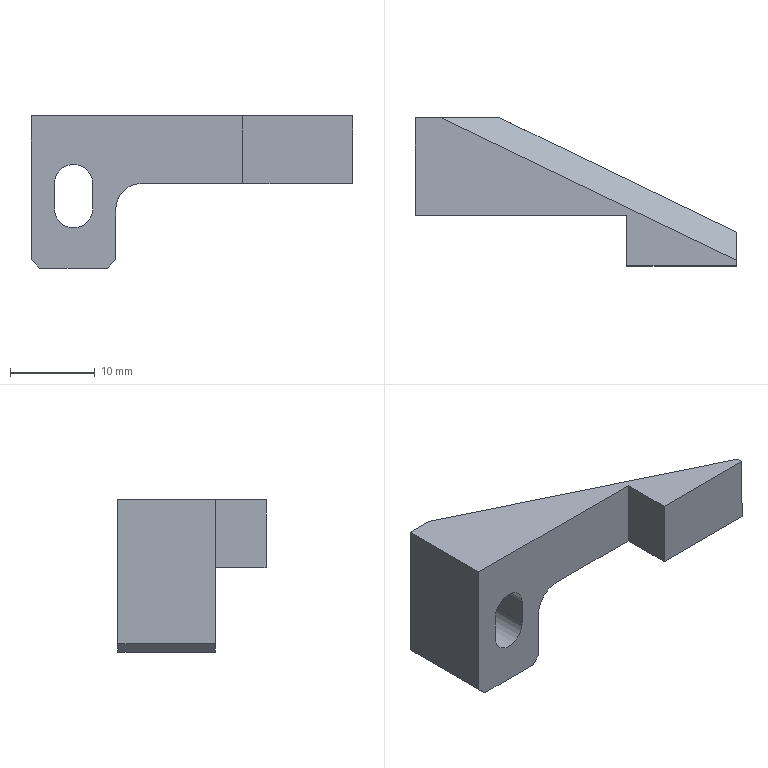Part | SolidWorks | features ICE 4, Chamfer 2, Extrusion 1, Fillet 1 | 1 solid | 25 faces | box 38 x 17.5 x 18 mm | volume 3099 mm3 | plane 19 | cylinder 6 | commonest cylinder face diameters 8 x3 4.5 x2 6 x1
STEP:
#1=CARTESIAN_POINT('',(5.,13.5,14.));
#2=VERTEX_POINT('',#1);
#3=CARTESIAN_POINT('',(9.,13.5,10.));
#4=VERTEX_POINT('',#3);
#5=CARTESIAN_POINT('',(5.,13.5,10.));
#6=DIRECTION('',(0.,1.,0.));
#7=DIRECTION('',(0.,0.,1.));
#8=AXIS2_PLACEMENT_3D('',#5,#6,#7);
#9=CIRCLE('',#8,4.);
#10=EDGE_CURVE('',#2,#4,#9,.T.);
#11=ORIENTED_EDGE('',*,*,#10,.F.);
#12=CARTESIAN_POINT('',(5.,17.5,14.));
#13=VERTEX_POINT('',#12);
#14=CARTESIAN_POINT('',(5.,13.5,14.));
#15=DIRECTION('',(0.,1.,0.));
#16=VECTOR('',#15,1000.);
#17=LINE('',#14,#16);
#18=EDGE_CURVE('',#2,#13,#17,.T.);
#19=ORIENTED_EDGE('',*,*,#18,.T.);
#20=CARTESIAN_POINT('',(9.,17.5,10.));
#21=VERTEX_POINT('',#20);
#22=CARTESIAN_POINT('',(5.,17.5,10.));
#23=DIRECTION('',(0.,1.,0.));
#24=DIRECTION('',(0.,0.,1.));
#25=AXIS2_PLACEMENT_3D('',#22,#23,#24);
#26=CIRCLE('',#25,4.);
#27=EDGE_CURVE('',#13,#21,#26,.T.);
#28=ORIENTED_EDGE('',*,*,#27,.T.);
#29=CARTESIAN_POINT('',(9.,13.5,10.));
#30=DIRECTION('',(0.,1.,0.));
#31=VECTOR('',#30,1000.);
#32=LINE('',#29,#31);
#33=EDGE_CURVE('',#4,#21,#32,.T.);
#34=ORIENTED_EDGE('',*,*,#33,.F.);
#35=EDGE_LOOP('',(#11,#19,#28,#34));
#36=FACE_OUTER_BOUND('',#35,.T.);
#37=CARTESIAN_POINT('',(5.,13.5,10.));
#38=DIRECTION('',(0.,1.,0.));
#39=DIRECTION('',(0.,0.,1.));
#40=AXIS2_PLACEMENT_3D('',#37,#38,#39);
#41=CYLINDRICAL_SURFACE('',#40,4.);
#42=ADVANCED_FACE('',(#36),#41,.F.);
#43=CARTESIAN_POINT('',(7.25,6.,10.));
#44=VERTEX_POINT('',#43);
#45=CARTESIAN_POINT('',(7.25,13.5,10.));
#46=VERTEX_POINT('',#45);
#47=CARTESIAN_POINT('',(7.25,-2.5,10.));
#48=DIRECTION('',(0.,1.,0.));
#49=VECTOR('',#48,1000.);
#50=LINE('',#47,#49);
#51=EDGE_CURVE('',#44,#46,#50,.T.);
#52=ORIENTED_EDGE('',*,*,#51,.F.);
#53=CARTESIAN_POINT('',(2.75,6.,10.));
#54=VERTEX_POINT('',#53);
#55=CARTESIAN_POINT('',(5.,6.,10.));
#56=DIRECTION('',(0.,-1.,0.));
#57=DIRECTION('',(0.,0.,1.));
#58=AXIS2_PLACEMENT_3D('',#55,#56,#57);
#59=CIRCLE('',#58,2.25);
#60=EDGE_CURVE('',#44,#54,#59,.T.);
#61=ORIENTED_EDGE('',*,*,#60,.T.);
#62=CARTESIAN_POINT('',(2.75,13.5,10.));
#63=VERTEX_POINT('',#62);
#64=CARTESIAN_POINT('',(2.75,-2.5,10.));
#65=DIRECTION('',(0.,1.,0.));
#66=VECTOR('',#65,1000.);
#67=LINE('',#64,#66);
#68=EDGE_CURVE('',#54,#63,#67,.T.);
#69=ORIENTED_EDGE('',*,*,#68,.T.);
#70=CARTESIAN_POINT('',(5.,13.5,10.));
#71=DIRECTION('',(0.,-1.,0.));
#72=DIRECTION('',(0.,0.,1.));
#73=AXIS2_PLACEMENT_3D('',#70,#71,#72);
#74=CIRCLE('',#73,2.25);
#75=EDGE_CURVE('',#46,#63,#74,.T.);
#76=ORIENTED_EDGE('',*,*,#75,.F.);
#77=EDGE_LOOP('',(#52,#61,#69,#76));
#78=FACE_OUTER_BOUND('',#77,.T.);
#79=CARTESIAN_POINT('',(5.,-2.5,10.));
#80=DIRECTION('',(0.,1.,0.));
#81=DIRECTION('',(-1.,0.,0.));
#82=AXIS2_PLACEMENT_3D('',#79,#80,#81);
#83=CYLINDRICAL_SURFACE('',#82,2.25);
#84=ADVANCED_FACE('',(#78),#83,.F.);
#85=ORIENTED_EDGE('',*,*,#68,.F.);
#86=CARTESIAN_POINT('',(2.75,6.,7.));
#87=VERTEX_POINT('',#86);
#88=CARTESIAN_POINT('',(2.75,6.,10.));
#89=DIRECTION('',(0.,0.,-1.));
#90=VECTOR('',#89,1000.);
#91=LINE('',#88,#90);
#92=EDGE_CURVE('',#54,#87,#91,.T.);
#93=ORIENTED_EDGE('',*,*,#92,.T.);
#94=CARTESIAN_POINT('',(2.75,13.5,7.));
#95=VERTEX_POINT('',#94);
#96=CARTESIAN_POINT('',(2.75,-2.5,7.));
#97=DIRECTION('',(0.,1.,0.));
#98=VECTOR('',#97,1000.);
#99=LINE('',#96,#98);
#100=EDGE_CURVE('',#87,#95,#99,.T.);
#101=ORIENTED_EDGE('',*,*,#100,.T.);
#102=CARTESIAN_POINT('',(2.75,13.5,10.));
#103=DIRECTION('',(0.,0.,-1.));
#104=VECTOR('',#103,1000.);
#105=LINE('',#102,#104);
#106=EDGE_CURVE('',#63,#95,#105,.T.);
#107=ORIENTED_EDGE('',*,*,#106,.F.);
#108=EDGE_LOOP('',(#85,#93,#101,#107));
#109=FACE_OUTER_BOUND('',#108,.T.);
#110=CARTESIAN_POINT('',(2.75,-2.5,10.));
#111=DIRECTION('',(-1.,0.,0.));
#112=DIRECTION('',(0.,-1.,0.));
#113=AXIS2_PLACEMENT_3D('',#110,#111,#112);
#114=PLANE('',#113);
#115=ADVANCED_FACE('',(#109),#114,.F.);
#116=ORIENTED_EDGE('',*,*,#100,.F.);
#117=CARTESIAN_POINT('',(7.25,6.,7.));
#118=VERTEX_POINT('',#117);
#119=CARTESIAN_POINT('',(5.,6.,7.));
#120=DIRECTION('',(0.,-1.,0.));
#121=DIRECTION('',(0.,0.,1.));
#122=AXIS2_PLACEMENT_3D('',#119,#120,#121);
#123=CIRCLE('',#122,2.25);
#124=EDGE_CURVE('',#87,#118,#123,.T.);
#125=ORIENTED_EDGE('',*,*,#124,.T.);
#126=CARTESIAN_POINT('',(7.25,13.5,7.));
#127=VERTEX_POINT('',#126);
#128=CARTESIAN_POINT('',(7.25,-2.5,7.));
#129=DIRECTION('',(0.,1.,0.));
#130=VECTOR('',#129,1000.);
#131=LINE('',#128,#130);
#132=EDGE_CURVE('',#118,#127,#131,.T.);
#133=ORIENTED_EDGE('',*,*,#132,.T.);
#134=CARTESIAN_POINT('',(5.,13.5,7.));
#135=DIRECTION('',(0.,-1.,0.));
#136=DIRECTION('',(0.,0.,1.));
#137=AXIS2_PLACEMENT_3D('',#134,#135,#136);
#138=CIRCLE('',#137,2.25);
#139=EDGE_CURVE('',#95,#127,#138,.T.);
#140=ORIENTED_EDGE('',*,*,#139,.F.);
#141=EDGE_LOOP('',(#116,#125,#133,#140));
#142=FACE_OUTER_BOUND('',#141,.T.);
#143=CARTESIAN_POINT('',(5.,-2.5,7.));
#144=DIRECTION('',(0.,1.,0.));
#145=DIRECTION('',(-1.,0.,0.));
#146=AXIS2_PLACEMENT_3D('',#143,#144,#145);
#147=CYLINDRICAL_SURFACE('',#146,2.25);
#148=ADVANCED_FACE('',(#142),#147,.F.);
#149=ORIENTED_EDGE('',*,*,#132,.F.);
#150=CARTESIAN_POINT('',(7.25,6.,10.));
#151=DIRECTION('',(0.,0.,1.));
#152=VECTOR('',#151,1000.);
#153=LINE('',#150,#152);
#154=EDGE_CURVE('',#118,#44,#153,.T.);
#155=ORIENTED_EDGE('',*,*,#154,.T.);
#156=ORIENTED_EDGE('',*,*,#51,.T.);
#157=CARTESIAN_POINT('',(7.25,13.5,10.));
#158=DIRECTION('',(0.,0.,1.));
#159=VECTOR('',#158,1000.);
#160=LINE('',#157,#159);
#161=EDGE_CURVE('',#127,#46,#160,.T.);
#162=ORIENTED_EDGE('',*,*,#161,.F.);
#163=EDGE_LOOP('',(#149,#155,#156,#162));
#164=FACE_OUTER_BOUND('',#163,.T.);
#165=CARTESIAN_POINT('',(7.25,-2.5,10.));
#166=DIRECTION('',(1.,0.,0.));
#167=DIRECTION('',(0.,1.,0.));
#168=AXIS2_PLACEMENT_3D('',#165,#166,#167);
#169=PLANE('',#168);
#170=ADVANCED_FACE('',(#164),#169,.F.);
#171=CARTESIAN_POINT('',(1.,17.5,7.));
#172=VERTEX_POINT('',#171);
#173=CARTESIAN_POINT('',(1.,17.5,10.));
#174=VERTEX_POINT('',#173);
#175=CARTESIAN_POINT('',(1.,17.5,7.));
#176=DIRECTION('',(0.,0.,1.));
#177=VECTOR('',#176,1000.);
#178=LINE('',#175,#177);
#179=EDGE_CURVE('',#172,#174,#178,.T.);
#180=ORIENTED_EDGE('',*,*,#179,.F.);
#181=CARTESIAN_POINT('',(9.,17.5,7.));
#182=VERTEX_POINT('',#181);
#183=CARTESIAN_POINT('',(5.,17.5,7.));
#184=DIRECTION('',(0.,1.,0.));
#185=DIRECTION('',(0.,0.,1.));
#186=AXIS2_PLACEMENT_3D('',#183,#184,#185);
#187=CIRCLE('',#186,4.);
#188=EDGE_CURVE('',#182,#172,#187,.T.);
#189=ORIENTED_EDGE('',*,*,#188,.F.);
#190=CARTESIAN_POINT('',(9.,17.5,7.));
#191=DIRECTION('',(0.,0.,-1.));
#192=VECTOR('',#191,1000.);
#193=LINE('',#190,#192);
#194=EDGE_CURVE('',#21,#182,#193,.T.);
#195=ORIENTED_EDGE('',*,*,#194,.F.);
#196=ORIENTED_EDGE('',*,*,#27,.F.);
#197=CARTESIAN_POINT('',(5.,17.5,10.));
#198=DIRECTION('',(0.,1.,0.));
#199=DIRECTION('',(0.,0.,1.));
#200=AXIS2_PLACEMENT_3D('',#197,#198,#199);
#201=CIRCLE('',#200,4.);
#202=EDGE_CURVE('',#174,#13,#201,.T.);
#203=ORIENTED_EDGE('',*,*,#202,.F.);
#204=EDGE_LOOP('',(#180,#189,#195,#196,#203));
#205=FACE_BOUND('',#204,.T.);
#206=CARTESIAN_POINT('',(9.,17.5,0.));
#207=VERTEX_POINT('',#206);
#208=CARTESIAN_POINT('',(1.,17.5,0.));
#209=VERTEX_POINT('',#208);
#210=CARTESIAN_POINT('',(10.,17.5,0.));
#211=DIRECTION('',(-1.,0.,0.));
#212=VECTOR('',#211,1000.);
#213=LINE('',#210,#212);
#214=EDGE_CURVE('',#207,#209,#213,.T.);
#215=ORIENTED_EDGE('',*,*,#214,.T.);
#216=CARTESIAN_POINT('',(0.,17.5,1.));
#217=VERTEX_POINT('',#216);
#218=CARTESIAN_POINT('',(0.,17.5,1.));
#219=DIRECTION('',(-0.7071,0.,0.7071));
#220=VECTOR('',#219,1000.);
#221=LINE('',#218,#220);
#222=EDGE_CURVE('',#209,#217,#221,.T.);
#223=ORIENTED_EDGE('',*,*,#222,.T.);
#224=CARTESIAN_POINT('',(0.,17.5,18.));
#225=VERTEX_POINT('',#224);
#226=CARTESIAN_POINT('',(0.,17.5,18.));
#227=DIRECTION('',(0.,0.,-1.));
#228=VECTOR('',#227,1000.);
#229=LINE('',#226,#228);
#230=EDGE_CURVE('',#225,#217,#229,.T.);
#231=ORIENTED_EDGE('',*,*,#230,.F.);
#232=CARTESIAN_POINT('',(3.092,17.5,18.));
#233=VERTEX_POINT('',#232);
#234=CARTESIAN_POINT('',(10.,17.5,18.));
#235=DIRECTION('',(-1.,0.,0.));
#236=VECTOR('',#235,1000.);
#237=LINE('',#234,#236);
#238=EDGE_CURVE('',#233,#225,#237,.T.);
#239=ORIENTED_EDGE('',*,*,#238,.F.);
#240=CARTESIAN_POINT('',(10.,17.5,15.));
#241=VERTEX_POINT('',#240);
#242=CARTESIAN_POINT('',(0.9814,17.5,18.917));
#243=DIRECTION('',(0.9172,0.,-0.3984));
#244=VECTOR('',#243,1000.);
#245=LINE('',#242,#244);
#246=EDGE_CURVE('',#233,#241,#245,.T.);
#247=ORIENTED_EDGE('',*,*,#246,.T.);
#248=CARTESIAN_POINT('',(10.,17.5,7.));
#249=VERTEX_POINT('',#248);
#250=CARTESIAN_POINT('',(10.,17.5,18.));
#251=DIRECTION('',(0.,0.,-1.));
#252=VECTOR('',#251,1000.);
#253=LINE('',#250,#252);
#254=EDGE_CURVE('',#241,#249,#253,.T.);
#255=ORIENTED_EDGE('',*,*,#254,.T.);
#256=CARTESIAN_POINT('',(10.,17.5,1.));
#257=VERTEX_POINT('',#256);
#258=CARTESIAN_POINT('',(10.,17.5,0.));
#259=DIRECTION('',(0.,0.,1.));
#260=VECTOR('',#259,1000.);
#261=LINE('',#258,#260);
#262=EDGE_CURVE('',#257,#249,#261,.T.);
#263=ORIENTED_EDGE('',*,*,#262,.F.);
#264=CARTESIAN_POINT('',(10.,17.5,1.));
#265=DIRECTION('',(-0.7071,0.,-0.7071));
#266=VECTOR('',#265,1000.);
#267=LINE('',#264,#266);
#268=EDGE_CURVE('',#257,#207,#267,.T.);
#269=ORIENTED_EDGE('',*,*,#268,.T.);
#270=EDGE_LOOP('',(#215,#223,#231,#239,#247,#255,#263,#269));
#271=FACE_OUTER_BOUND('',#270,.T.);
#272=CARTESIAN_POINT('',(10.,17.5,18.));
#273=DIRECTION('',(0.,-1.,0.));
#274=DIRECTION('',(1.,0.,0.));
#275=AXIS2_PLACEMENT_3D('',#272,#273,#274);
#276=PLANE('',#275);
#277=ADVANCED_FACE('',(#205,#271),#276,.F.);
#278=ORIENTED_EDGE('',*,*,#230,.T.);
#279=CARTESIAN_POINT('',(0.,6.,1.));
#280=VERTEX_POINT('',#279);
#281=CARTESIAN_POINT('',(0.,17.5,1.));
#282=DIRECTION('',(0.,-1.,0.));
#283=VECTOR('',#282,1000.);
#284=LINE('',#281,#283);
#285=EDGE_CURVE('',#217,#280,#284,.T.);
#286=ORIENTED_EDGE('',*,*,#285,.T.);
#287=CARTESIAN_POINT('',(0.,6.,18.));
#288=VERTEX_POINT('',#287);
#289=CARTESIAN_POINT('',(0.,6.,0.));
#290=DIRECTION('',(0.,0.,1.));
#291=VECTOR('',#290,1000.);
#292=LINE('',#289,#291);
#293=EDGE_CURVE('',#280,#288,#292,.T.);
#294=ORIENTED_EDGE('',*,*,#293,.T.);
#295=CARTESIAN_POINT('',(0.,17.5,18.));
#296=DIRECTION('',(0.,-1.,0.));
#297=VECTOR('',#296,1000.);
#298=LINE('',#295,#297);
#299=EDGE_CURVE('',#225,#288,#298,.T.);
#300=ORIENTED_EDGE('',*,*,#299,.F.);
#301=EDGE_LOOP('',(#278,#286,#294,#300));
#302=FACE_OUTER_BOUND('',#301,.T.);
#303=CARTESIAN_POINT('',(0.,17.5,18.));
#304=DIRECTION('',(1.,0.,0.));
#305=DIRECTION('',(0.,1.,0.));
#306=AXIS2_PLACEMENT_3D('',#303,#304,#305);
#307=PLANE('',#306);
#308=ADVANCED_FACE('',(#302),#307,.F.);
#309=CARTESIAN_POINT('',(25.,0.,10.));
#310=VERTEX_POINT('',#309);
#311=CARTESIAN_POINT('',(25.,0.,18.));
#312=VERTEX_POINT('',#311);
#313=CARTESIAN_POINT('',(25.,0.,0.));
#314=DIRECTION('',(0.,0.,1.));
#315=VECTOR('',#314,1000.);
#316=LINE('',#313,#315);
#317=EDGE_CURVE('',#310,#312,#316,.T.);
#318=ORIENTED_EDGE('',*,*,#317,.F.);
#319=CARTESIAN_POINT('',(38.,0.,10.));
#320=VERTEX_POINT('',#319);
#321=CARTESIAN_POINT('',(38.,0.,10.));
#322=DIRECTION('',(1.,0.,0.));
#323=VECTOR('',#322,1000.);
#324=LINE('',#321,#323);
#325=EDGE_CURVE('',#310,#320,#324,.T.);
#326=ORIENTED_EDGE('',*,*,#325,.T.);
#327=CARTESIAN_POINT('',(38.,0.,18.));
#328=VERTEX_POINT('',#327);
#329=CARTESIAN_POINT('',(38.,0.,18.));
#330=DIRECTION('',(0.,0.,-1.));
#331=VECTOR('',#330,1000.);
#332=LINE('',#329,#331);
#333=EDGE_CURVE('',#328,#320,#332,.T.);
#334=ORIENTED_EDGE('',*,*,#333,.F.);
#335=CARTESIAN_POINT('',(0.,0.,18.));
#336=DIRECTION('',(1.,0.,0.));
#337=VECTOR('',#336,1000.);
#338=LINE('',#335,#337);
#339=EDGE_CURVE('',#312,#328,#338,.T.);
#340=ORIENTED_EDGE('',*,*,#339,.F.);
#341=EDGE_LOOP('',(#318,#326,#334,#340));
#342=FACE_OUTER_BOUND('',#341,.T.);
#343=CARTESIAN_POINT('',(0.,0.,18.));
#344=DIRECTION('',(0.,1.,0.));
#345=DIRECTION('',(0.,0.,1.));
#346=AXIS2_PLACEMENT_3D('',#343,#344,#345);
#347=PLANE('',#346);
#348=ADVANCED_FACE('',(#342),#347,.F.);
#349=ORIENTED_EDGE('',*,*,#333,.T.);
#350=CARTESIAN_POINT('',(38.,4.,10.));
#351=VERTEX_POINT('',#350);
#352=CARTESIAN_POINT('',(38.,0.,10.));
#353=DIRECTION('',(0.,1.,0.));
#354=VECTOR('',#353,1000.);
#355=LINE('',#352,#354);
#356=EDGE_CURVE('',#320,#351,#355,.T.);
#357=ORIENTED_EDGE('',*,*,#356,.T.);
#358=CARTESIAN_POINT('',(38.,4.,15.));
#359=VERTEX_POINT('',#358);
#360=CARTESIAN_POINT('',(38.,4.,18.));
#361=DIRECTION('',(0.,0.,-1.));
#362=VECTOR('',#361,1000.);
#363=LINE('',#360,#362);
#364=EDGE_CURVE('',#359,#351,#363,.T.);
#365=ORIENTED_EDGE('',*,*,#364,.F.);
#366=CARTESIAN_POINT('',(38.,0.6695,18.));
#367=VERTEX_POINT('',#366);
#368=CARTESIAN_POINT('',(38.,10.629,9.029));
#369=DIRECTION('',(0.,-0.743,0.6693));
#370=VECTOR('',#369,1000.);
#371=LINE('',#368,#370);
#372=EDGE_CURVE('',#359,#367,#371,.T.);
#373=ORIENTED_EDGE('',*,*,#372,.T.);
#374=CARTESIAN_POINT('',(38.,0.,18.));
#375=DIRECTION('',(0.,1.,0.));
#376=VECTOR('',#375,1000.);
#377=LINE('',#374,#376);
#378=EDGE_CURVE('',#328,#367,#377,.T.);
#379=ORIENTED_EDGE('',*,*,#378,.F.);
#380=EDGE_LOOP('',(#349,#357,#365,#373,#379));
#381=FACE_OUTER_BOUND('',#380,.T.);
#382=CARTESIAN_POINT('',(38.,0.,18.));
#383=DIRECTION('',(-1.,0.,0.));
#384=DIRECTION('',(0.,0.,1.));
#385=AXIS2_PLACEMENT_3D('',#382,#383,#384);
#386=PLANE('',#385);
#387=ADVANCED_FACE('',(#381),#386,.F.);
#388=ORIENTED_EDGE('',*,*,#364,.T.);
#389=CARTESIAN_POINT('',(13.,16.054,10.));
#390=VERTEX_POINT('',#389);
#391=CARTESIAN_POINT('',(38.,4.,10.));
#392=DIRECTION('',(-0.9008,0.4343,0.));
#393=VECTOR('',#392,1000.);
#394=LINE('',#391,#393);
#395=EDGE_CURVE('',#351,#390,#394,.T.);
#396=ORIENTED_EDGE('',*,*,#395,.T.);
#397=CARTESIAN_POINT('',(13.,16.054,10.));
#398=CARTESIAN_POINT('',(11.243,16.901,10.));
#399=CARTESIAN_POINT('',(10.,17.5,8.757));
#400=CARTESIAN_POINT('',(10.,17.5,7.));
#401=(BOUNDED_CURVE()B_SPLINE_CURVE(3,(#397,#398,#399,#400),.UNSPECIFIED.,.F.,.F.)B_SPLINE_CURVE_WITH_KNOTS((4,4),(1.571,3.142),.UNSPECIFIED.)CURVE()GEOMETRIC_REPRESENTATION_ITEM()RATIONAL_B_SPLINE_CURVE((1.,0.8047,0.8047,1.))REPRESENTATION_ITEM(''));
#402=EDGE_CURVE('',#390,#249,#401,.T.);
#403=ORIENTED_EDGE('',*,*,#402,.T.);
#404=ORIENTED_EDGE('',*,*,#254,.F.);
#405=CARTESIAN_POINT('',(38.,4.,15.));
#406=DIRECTION('',(0.9008,-0.4343,0.));
#407=VECTOR('',#406,1000.);
#408=LINE('',#405,#407);
#409=EDGE_CURVE('',#241,#359,#408,.T.);
#410=ORIENTED_EDGE('',*,*,#409,.T.);
#411=EDGE_LOOP('',(#388,#396,#403,#404,#410));
#412=FACE_OUTER_BOUND('',#411,.T.);
#413=CARTESIAN_POINT('',(38.,4.,18.));
#414=DIRECTION('',(-0.4343,-0.9008,0.));
#415=DIRECTION('',(0.9008,-0.4343,0.));
#416=AXIS2_PLACEMENT_3D('',#413,#414,#415);
#417=PLANE('',#416);
#418=ADVANCED_FACE('',(#412),#417,.F.);
#419=CARTESIAN_POINT('',(25.,6.,18.));
#420=VERTEX_POINT('',#419);
#421=CARTESIAN_POINT('',(0.,6.,18.));
#422=DIRECTION('',(-1.,0.,0.));
#423=VECTOR('',#422,1000.);
#424=LINE('',#421,#423);
#425=EDGE_CURVE('',#420,#288,#424,.T.);
#426=ORIENTED_EDGE('',*,*,#425,.F.);
#427=CARTESIAN_POINT('',(25.,0.,18.));
#428=DIRECTION('',(0.,1.,0.));
#429=VECTOR('',#428,1000.);
#430=LINE('',#427,#429);
#431=EDGE_CURVE('',#312,#420,#430,.T.);
#432=ORIENTED_EDGE('',*,*,#431,.F.);
#433=ORIENTED_EDGE('',*,*,#339,.T.);
#434=ORIENTED_EDGE('',*,*,#378,.T.);
#435=CARTESIAN_POINT('',(8.697,14.798,18.));
#436=DIRECTION('',(-0.9008,0.4343,0.));
#437=VECTOR('',#436,1000.);
#438=LINE('',#435,#437);
#439=EDGE_CURVE('',#367,#233,#438,.T.);
#440=ORIENTED_EDGE('',*,*,#439,.T.);
#441=ORIENTED_EDGE('',*,*,#238,.T.);
#442=ORIENTED_EDGE('',*,*,#299,.T.);
#443=EDGE_LOOP('',(#426,#432,#433,#434,#440,#441,#442));
#444=FACE_OUTER_BOUND('',#443,.T.);
#445=CARTESIAN_POINT('',(0.,17.5,18.));
#446=DIRECTION('',(0.,0.,1.));
#447=DIRECTION('',(1.,0.,0.));
#448=AXIS2_PLACEMENT_3D('',#445,#446,#447);
#449=PLANE('',#448);
#450=ADVANCED_FACE('',(#444),#449,.T.);
#451=CARTESIAN_POINT('',(9.,6.,0.));
#452=VERTEX_POINT('',#451);
#453=CARTESIAN_POINT('',(1.,6.,0.));
#454=VERTEX_POINT('',#453);
#455=CARTESIAN_POINT('',(0.,6.,0.));
#456=DIRECTION('',(-1.,0.,0.));
#457=VECTOR('',#456,1000.);
#458=LINE('',#455,#457);
#459=EDGE_CURVE('',#452,#454,#458,.T.);
#460=ORIENTED_EDGE('',*,*,#459,.T.);
#461=CARTESIAN_POINT('',(1.,17.5,0.));
#462=DIRECTION('',(0.,1.,0.));
#463=VECTOR('',#462,1000.);
#464=LINE('',#461,#463);
#465=EDGE_CURVE('',#454,#209,#464,.T.);
#466=ORIENTED_EDGE('',*,*,#465,.T.);
#467=ORIENTED_EDGE('',*,*,#214,.F.);
#468=CARTESIAN_POINT('',(9.,17.5,0.));
#469=DIRECTION('',(0.,-1.,0.));
#470=VECTOR('',#469,1000.);
#471=LINE('',#468,#470);
#472=EDGE_CURVE('',#207,#452,#471,.T.);
#473=ORIENTED_EDGE('',*,*,#472,.T.);
#474=EDGE_LOOP('',(#460,#466,#467,#473));
#475=FACE_OUTER_BOUND('',#474,.T.);
#476=CARTESIAN_POINT('',(0.,17.5,0.));
#477=DIRECTION('',(0.,0.,1.));
#478=DIRECTION('',(1.,0.,0.));
#479=AXIS2_PLACEMENT_3D('',#476,#477,#478);
#480=PLANE('',#479);
#481=ADVANCED_FACE('',(#475),#480,.F.);
#482=ORIENTED_EDGE('',*,*,#372,.F.);
#483=ORIENTED_EDGE('',*,*,#409,.F.);
#484=ORIENTED_EDGE('',*,*,#246,.F.);
#485=ORIENTED_EDGE('',*,*,#439,.F.);
#486=EDGE_LOOP('',(#482,#483,#484,#485));
#487=FACE_OUTER_BOUND('',#486,.T.);
#488=CARTESIAN_POINT('',(0.5833,18.71,18.));
#489=DIRECTION('',(0.3071,0.6369,0.7071));
#490=DIRECTION('',(0.,-0.743,0.6693));
#491=AXIS2_PLACEMENT_3D('',#488,#489,#490);
#492=PLANE('',#491);
#493=ADVANCED_FACE('',(#487),#492,.T.);
#494=CARTESIAN_POINT('',(9.,13.5,7.));
#495=VERTEX_POINT('',#494);
#496=CARTESIAN_POINT('',(1.,13.5,7.));
#497=VERTEX_POINT('',#496);
#498=CARTESIAN_POINT('',(5.,13.5,7.));
#499=DIRECTION('',(0.,1.,0.));
#500=DIRECTION('',(0.,0.,1.));
#501=AXIS2_PLACEMENT_3D('',#498,#499,#500);
#502=CIRCLE('',#501,4.);
#503=EDGE_CURVE('',#495,#497,#502,.T.);
#504=ORIENTED_EDGE('',*,*,#503,.T.);
#505=CARTESIAN_POINT('',(1.,13.5,10.));
#506=VERTEX_POINT('',#505);
#507=CARTESIAN_POINT('',(1.,13.5,7.));
#508=DIRECTION('',(0.,0.,1.));
#509=VECTOR('',#508,1000.);
#510=LINE('',#507,#509);
#511=EDGE_CURVE('',#497,#506,#510,.T.);
#512=ORIENTED_EDGE('',*,*,#511,.T.);
#513=CARTESIAN_POINT('',(5.,13.5,10.));
#514=DIRECTION('',(0.,1.,0.));
#515=DIRECTION('',(0.,0.,1.));
#516=AXIS2_PLACEMENT_3D('',#513,#514,#515);
#517=CIRCLE('',#516,4.);
#518=EDGE_CURVE('',#506,#2,#517,.T.);
#519=ORIENTED_EDGE('',*,*,#518,.T.);
#520=ORIENTED_EDGE('',*,*,#10,.T.);
#521=CARTESIAN_POINT('',(9.,13.5,7.));
#522=DIRECTION('',(0.,0.,-1.));
#523=VECTOR('',#522,1000.);
#524=LINE('',#521,#523);
#525=EDGE_CURVE('',#4,#495,#524,.T.);
#526=ORIENTED_EDGE('',*,*,#525,.T.);
#527=EDGE_LOOP('',(#504,#512,#519,#520,#526));
#528=FACE_OUTER_BOUND('',#527,.T.);
#529=ORIENTED_EDGE('',*,*,#75,.T.);
#530=ORIENTED_EDGE('',*,*,#106,.T.);
#531=ORIENTED_EDGE('',*,*,#139,.T.);
#532=ORIENTED_EDGE('',*,*,#161,.T.);
#533=EDGE_LOOP('',(#529,#530,#531,#532));
#534=FACE_BOUND('',#533,.T.);
#535=CARTESIAN_POINT('',(5.,13.5,7.));
#536=DIRECTION('',(0.,1.,0.));
#537=DIRECTION('',(0.,0.,1.));
#538=AXIS2_PLACEMENT_3D('',#535,#536,#537);
#539=PLANE('',#538);
#540=ADVANCED_FACE('',(#528,#534),#539,.T.);
#541=ORIENTED_EDGE('',*,*,#188,.T.);
#542=CARTESIAN_POINT('',(1.,13.5,7.));
#543=DIRECTION('',(0.,1.,0.));
#544=VECTOR('',#543,1000.);
#545=LINE('',#542,#544);
#546=EDGE_CURVE('',#497,#172,#545,.T.);
#547=ORIENTED_EDGE('',*,*,#546,.F.);
#548=ORIENTED_EDGE('',*,*,#503,.F.);
#549=CARTESIAN_POINT('',(9.,13.5,7.));
#550=DIRECTION('',(0.,1.,0.));
#551=VECTOR('',#550,1000.);
#552=LINE('',#549,#551);
#553=EDGE_CURVE('',#495,#182,#552,.T.);
#554=ORIENTED_EDGE('',*,*,#553,.T.);
#555=EDGE_LOOP('',(#541,#547,#548,#554));
#556=FACE_OUTER_BOUND('',#555,.T.);
#557=CARTESIAN_POINT('',(5.,13.5,7.));
#558=DIRECTION('',(0.,1.,0.));
#559=DIRECTION('',(0.,0.,1.));
#560=AXIS2_PLACEMENT_3D('',#557,#558,#559);
#561=CYLINDRICAL_SURFACE('',#560,4.);
#562=ADVANCED_FACE('',(#556),#561,.F.);
#563=ORIENTED_EDGE('',*,*,#194,.T.);
#564=ORIENTED_EDGE('',*,*,#553,.F.);
#565=ORIENTED_EDGE('',*,*,#525,.F.);
#566=ORIENTED_EDGE('',*,*,#33,.T.);
#567=EDGE_LOOP('',(#563,#564,#565,#566));
#568=FACE_OUTER_BOUND('',#567,.T.);
#569=CARTESIAN_POINT('',(9.,13.5,7.));
#570=DIRECTION('',(1.,0.,0.));
#571=DIRECTION('',(0.,0.,-1.));
#572=AXIS2_PLACEMENT_3D('',#569,#570,#571);
#573=PLANE('',#572);
#574=ADVANCED_FACE('',(#568),#573,.F.);
#575=ORIENTED_EDGE('',*,*,#18,.F.);
#576=ORIENTED_EDGE('',*,*,#518,.F.);
#577=CARTESIAN_POINT('',(1.,13.5,10.));
#578=DIRECTION('',(0.,1.,0.));
#579=VECTOR('',#578,1000.);
#580=LINE('',#577,#579);
#581=EDGE_CURVE('',#506,#174,#580,.T.);
#582=ORIENTED_EDGE('',*,*,#581,.T.);
#583=ORIENTED_EDGE('',*,*,#202,.T.);
#584=EDGE_LOOP('',(#575,#576,#582,#583));
#585=FACE_OUTER_BOUND('',#584,.T.);
#586=CARTESIAN_POINT('',(5.,13.5,10.));
#587=DIRECTION('',(0.,1.,0.));
#588=DIRECTION('',(0.,0.,1.));
#589=AXIS2_PLACEMENT_3D('',#586,#587,#588);
#590=CYLINDRICAL_SURFACE('',#589,4.);
#591=ADVANCED_FACE('',(#585),#590,.F.);
#592=ORIENTED_EDGE('',*,*,#179,.T.);
#593=ORIENTED_EDGE('',*,*,#581,.F.);
#594=ORIENTED_EDGE('',*,*,#511,.F.);
#595=ORIENTED_EDGE('',*,*,#546,.T.);
#596=EDGE_LOOP('',(#592,#593,#594,#595));
#597=FACE_OUTER_BOUND('',#596,.T.);
#598=CARTESIAN_POINT('',(1.,13.5,7.));
#599=DIRECTION('',(-1.,0.,0.));
#600=DIRECTION('',(0.,0.,1.));
#601=AXIS2_PLACEMENT_3D('',#598,#599,#600);
#602=PLANE('',#601);
#603=ADVANCED_FACE('',(#597),#602,.F.);
#604=ORIENTED_EDGE('',*,*,#293,.F.);
#605=CARTESIAN_POINT('',(0.,6.,1.));
#606=DIRECTION('',(0.7071,0.,-0.7071));
#607=VECTOR('',#606,1000.);
#608=LINE('',#605,#607);
#609=EDGE_CURVE('',#280,#454,#608,.T.);
#610=ORIENTED_EDGE('',*,*,#609,.T.);
#611=ORIENTED_EDGE('',*,*,#459,.F.);
#612=CARTESIAN_POINT('',(10.,6.,1.));
#613=VERTEX_POINT('',#612);
#614=CARTESIAN_POINT('',(10.,6.,1.));
#615=DIRECTION('',(0.7071,0.,0.7071));
#616=VECTOR('',#615,1000.);
#617=LINE('',#614,#616);
#618=EDGE_CURVE('',#452,#613,#617,.T.);
#619=ORIENTED_EDGE('',*,*,#618,.T.);
#620=CARTESIAN_POINT('',(10.,6.,7.));
#621=VERTEX_POINT('',#620);
#622=CARTESIAN_POINT('',(10.,6.,0.));
#623=DIRECTION('',(0.,0.,1.));
#624=VECTOR('',#623,1000.);
#625=LINE('',#622,#624);
#626=EDGE_CURVE('',#613,#621,#625,.T.);
#627=ORIENTED_EDGE('',*,*,#626,.T.);
#628=CARTESIAN_POINT('',(13.,6.,10.));
#629=VERTEX_POINT('',#628);
#630=CARTESIAN_POINT('',(13.,6.,7.));
#631=DIRECTION('',(0.,1.,0.));
#632=DIRECTION('',(0.,0.,1.));
#633=AXIS2_PLACEMENT_3D('',#630,#631,#632);
#634=CIRCLE('',#633,3.);
#635=EDGE_CURVE('',#621,#629,#634,.T.);
#636=ORIENTED_EDGE('',*,*,#635,.T.);
#637=CARTESIAN_POINT('',(25.,6.,10.));
#638=VERTEX_POINT('',#637);
#639=CARTESIAN_POINT('',(0.,6.,10.));
#640=DIRECTION('',(1.,0.,0.));
#641=VECTOR('',#640,1000.);
#642=LINE('',#639,#641);
#643=EDGE_CURVE('',#629,#638,#642,.T.);
#644=ORIENTED_EDGE('',*,*,#643,.T.);
#645=CARTESIAN_POINT('',(25.,6.,0.));
#646=DIRECTION('',(0.,0.,1.));
#647=VECTOR('',#646,1000.);
#648=LINE('',#645,#647);
#649=EDGE_CURVE('',#638,#420,#648,.T.);
#650=ORIENTED_EDGE('',*,*,#649,.T.);
#651=ORIENTED_EDGE('',*,*,#425,.T.);
#652=EDGE_LOOP('',(#604,#610,#611,#619,#627,#636,#644,#650,#651));
#653=FACE_OUTER_BOUND('',#652,.T.);
#654=ORIENTED_EDGE('',*,*,#154,.F.);
#655=ORIENTED_EDGE('',*,*,#124,.F.);
#656=ORIENTED_EDGE('',*,*,#92,.F.);
#657=ORIENTED_EDGE('',*,*,#60,.F.);
#658=EDGE_LOOP('',(#654,#655,#656,#657));
#659=FACE_BOUND('',#658,.T.);
#660=CARTESIAN_POINT('',(0.,6.,0.));
#661=DIRECTION('',(0.,1.,0.));
#662=DIRECTION('',(0.,0.,1.));
#663=AXIS2_PLACEMENT_3D('',#660,#661,#662);
#664=PLANE('',#663);
#665=ADVANCED_FACE('',(#653,#659),#664,.F.);
#666=ORIENTED_EDGE('',*,*,#649,.F.);
#667=CARTESIAN_POINT('',(25.,0.,10.));
#668=DIRECTION('',(0.,-1.,0.));
#669=VECTOR('',#668,1000.);
#670=LINE('',#667,#669);
#671=EDGE_CURVE('',#638,#310,#670,.T.);
#672=ORIENTED_EDGE('',*,*,#671,.T.);
#673=ORIENTED_EDGE('',*,*,#317,.T.);
#674=ORIENTED_EDGE('',*,*,#431,.T.);
#675=EDGE_LOOP('',(#666,#672,#673,#674));
#676=FACE_OUTER_BOUND('',#675,.T.);
#677=CARTESIAN_POINT('',(25.,0.,0.));
#678=DIRECTION('',(1.,0.,0.));
#679=DIRECTION('',(0.,0.,-1.));
#680=AXIS2_PLACEMENT_3D('',#677,#678,#679);
#681=PLANE('',#680);
#682=ADVANCED_FACE('',(#676),#681,.F.);
#683=ORIENTED_EDGE('',*,*,#626,.F.);
#684=CARTESIAN_POINT('',(10.,0.,1.));
#685=DIRECTION('',(0.,1.,0.));
#686=VECTOR('',#685,1000.);
#687=LINE('',#684,#686);
#688=EDGE_CURVE('',#613,#257,#687,.T.);
#689=ORIENTED_EDGE('',*,*,#688,.T.);
#690=ORIENTED_EDGE('',*,*,#262,.T.);
#691=CARTESIAN_POINT('',(10.,6.,7.));
#692=DIRECTION('',(0.,-1.,0.));
#693=VECTOR('',#692,1000.);
#694=LINE('',#691,#693);
#695=EDGE_CURVE('',#249,#621,#694,.T.);
#696=ORIENTED_EDGE('',*,*,#695,.T.);
#697=EDGE_LOOP('',(#683,#689,#690,#696));
#698=FACE_OUTER_BOUND('',#697,.T.);
#699=CARTESIAN_POINT('',(10.,0.,0.));
#700=DIRECTION('',(-1.,0.,0.));
#701=DIRECTION('',(0.,-1.,0.));
#702=AXIS2_PLACEMENT_3D('',#699,#700,#701);
#703=PLANE('',#702);
#704=ADVANCED_FACE('',(#698),#703,.F.);
#705=ORIENTED_EDGE('',*,*,#643,.F.);
#706=CARTESIAN_POINT('',(13.,17.5,10.));
#707=DIRECTION('',(0.,1.,0.));
#708=VECTOR('',#707,1000.);
#709=LINE('',#706,#708);
#710=EDGE_CURVE('',#629,#390,#709,.T.);
#711=ORIENTED_EDGE('',*,*,#710,.T.);
#712=ORIENTED_EDGE('',*,*,#395,.F.);
#713=ORIENTED_EDGE('',*,*,#356,.F.);
#714=ORIENTED_EDGE('',*,*,#325,.F.);
#715=ORIENTED_EDGE('',*,*,#671,.F.);
#716=EDGE_LOOP('',(#705,#711,#712,#713,#714,#715));
#717=FACE_OUTER_BOUND('',#716,.T.);
#718=CARTESIAN_POINT('',(38.,0.,10.));
#719=DIRECTION('',(0.,0.,1.));
#720=DIRECTION('',(1.,0.,0.));
#721=AXIS2_PLACEMENT_3D('',#718,#719,#720);
#722=PLANE('',#721);
#723=ADVANCED_FACE('',(#717),#722,.F.);
#724=ORIENTED_EDGE('',*,*,#635,.F.);
#725=ORIENTED_EDGE('',*,*,#695,.F.);
#726=ORIENTED_EDGE('',*,*,#402,.F.);
#727=ORIENTED_EDGE('',*,*,#710,.F.);
#728=EDGE_LOOP('',(#724,#725,#726,#727));
#729=FACE_OUTER_BOUND('',#728,.T.);
#730=CARTESIAN_POINT('',(13.,0.,7.));
#731=DIRECTION('',(0.,-1.,0.));
#732=DIRECTION('',(1.,0.,0.));
#733=AXIS2_PLACEMENT_3D('',#730,#731,#732);
#734=CYLINDRICAL_SURFACE('',#733,3.);
#735=ADVANCED_FACE('',(#729),#734,.F.);
#736=ORIENTED_EDGE('',*,*,#222,.F.);
#737=ORIENTED_EDGE('',*,*,#465,.F.);
#738=ORIENTED_EDGE('',*,*,#609,.F.);
#739=ORIENTED_EDGE('',*,*,#285,.F.);
#740=EDGE_LOOP('',(#736,#737,#738,#739));
#741=FACE_OUTER_BOUND('',#740,.T.);
#742=CARTESIAN_POINT('',(0.,17.5,1.));
#743=DIRECTION('',(0.7071,0.,0.7071));
#744=DIRECTION('',(0.,-1.,0.));
#745=AXIS2_PLACEMENT_3D('',#742,#743,#744);
#746=PLANE('',#745);
#747=ADVANCED_FACE('',(#741),#746,.F.);
#748=ORIENTED_EDGE('',*,*,#618,.F.);
#749=ORIENTED_EDGE('',*,*,#472,.F.);
#750=ORIENTED_EDGE('',*,*,#268,.F.);
#751=ORIENTED_EDGE('',*,*,#688,.F.);
#752=EDGE_LOOP('',(#748,#749,#750,#751));
#753=FACE_OUTER_BOUND('',#752,.T.);
#754=CARTESIAN_POINT('',(10.,0.,1.));
#755=DIRECTION('',(-0.7071,0.,0.7071));
#756=DIRECTION('',(0.,1.,0.));
#757=AXIS2_PLACEMENT_3D('',#754,#755,#756);
#758=PLANE('',#757);
#759=ADVANCED_FACE('',(#753),#758,.F.);
#760=CLOSED_SHELL('',(#42,#84,#115,#148,#170,#277,#308,#348,#387,#418,#450,#481,#493,#540,#562,#574,#591,#603,#665,#682,#704,#723,#735,#747,#759));
#761=MANIFOLD_SOLID_BREP('',#760);
#762=CARTESIAN_POINT('',(0.,0.,0.));
#763=DIRECTION('',(0.,0.,1.));
#764=DIRECTION('',(1.,0.,0.));
#765=AXIS2_PLACEMENT_3D('',#762,#763,#764);
#766=(LENGTH_UNIT()NAMED_UNIT(*)SI_UNIT(.MILLI.,.METRE.));
#767=UNCERTAINTY_MEASURE_WITH_UNIT(LENGTH_MEASURE(0.00001),#766,'','');
#768=(NAMED_UNIT(*)PLANE_ANGLE_UNIT()SI_UNIT($,.RADIAN.));
#769=(NAMED_UNIT(*)SI_UNIT($,.STERADIAN.)SOLID_ANGLE_UNIT());
#770=(GEOMETRIC_REPRESENTATION_CONTEXT(3)GLOBAL_UNCERTAINTY_ASSIGNED_CONTEXT((#767))GLOBAL_UNIT_ASSIGNED_CONTEXT((#766,#768,#769))REPRESENTATION_CONTEXT('',''));
#771=ADVANCED_BREP_SHAPE_REPRESENTATION('',(#761,#765),#770);